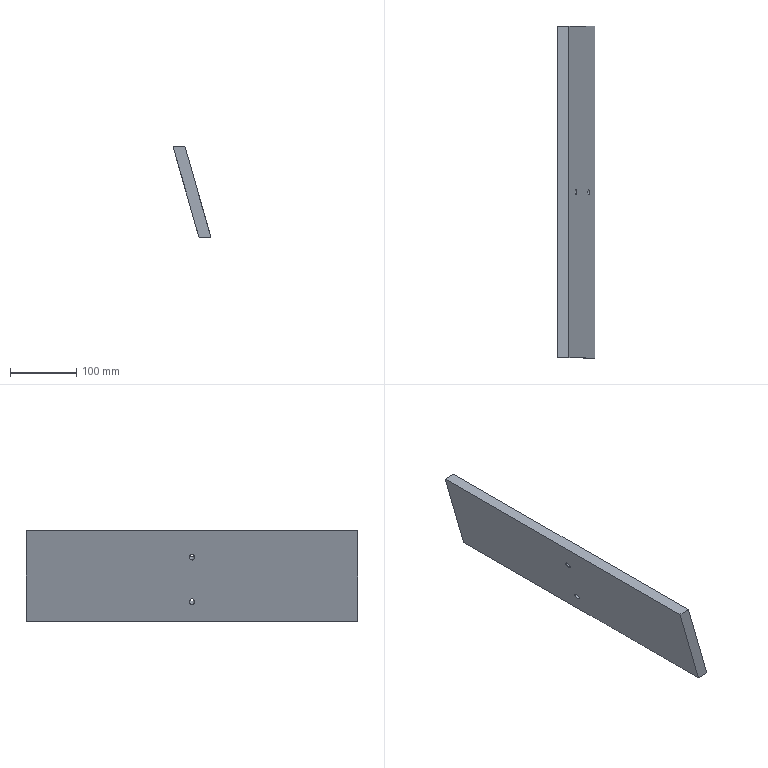Part | STEP file | Frame_top | 1 solid | 8 faces | box 57.278 x 502 x 136.98 mm | volume 1235548 mm3 | plane 6 | cylinder 2 | commonest cylinder face diameters 9 x2
STEP:
#1=CARTESIAN_POINT('',(0.,0.,0.));
#2=DIRECTION('',(0.,0.,1.));
#3=DIRECTION('',(1.,0.,0.));
#4=AXIS2_PLACEMENT_3D('',#1,#2,#3);
#5=CARTESIAN_POINT('',(-29.43,251.,71.25));
#6=VERTEX_POINT('',#5);
#7=CARTESIAN_POINT('',(-29.43,-251.,71.25));
#8=VERTEX_POINT('',#7);
#9=CARTESIAN_POINT('',(-29.43,251.,71.25));
#10=DIRECTION('',(0.,-1.,0.));
#11=VECTOR('',#10,1.);
#12=LINE('',#9,#11);
#13=CARTESIAN_POINT('',(-29.43,251.,71.25));
#14=DIRECTION('',(0.,0.,1.));
#15=DIRECTION('',(1.,0.,0.));
#16=AXIS2_PLACEMENT_3D('',#13,#14,#15);
#17=PLANE('',#16);
#18=CARTESIAN_POINT('',(0.,0.));
#19=DIRECTION('',(0.,-1.));
#20=VECTOR('',#19,1.);
#21=LINE('',#18,#20);
#22=(GEOMETRIC_REPRESENTATION_CONTEXT(2)PARAMETRIC_REPRESENTATION_CONTEXT()REPRESENTATION_CONTEXT('',''));
#23=DEFINITIONAL_REPRESENTATION('',(#21),#22);
#24=PCURVE('',#17,#23);
#25=CARTESIAN_POINT('',(9.848,251.,-65.73));
#26=DIRECTION('',(-0.9613,0.,-0.2756));
#27=DIRECTION('',(-0.2756,0.,0.9613));
#28=AXIS2_PLACEMENT_3D('',#25,#26,#27);
#29=PLANE('',#28);
#30=CARTESIAN_POINT('',(142.5,0.));
#31=DIRECTION('',(0.,-1.));
#32=VECTOR('',#31,1.);
#33=LINE('',#30,#32);
#34=(GEOMETRIC_REPRESENTATION_CONTEXT(2)PARAMETRIC_REPRESENTATION_CONTEXT()REPRESENTATION_CONTEXT('',''));
#35=DEFINITIONAL_REPRESENTATION('',(#33),#34);
#36=PCURVE('',#29,#35);
#37=SURFACE_CURVE('',#12,(#24,#36),.PCURVE_S1.);
#38=EDGE_CURVE('',#6,#8,#37,.T.);
#39=ORIENTED_EDGE('',*,*,#38,.T.);
#40=CARTESIAN_POINT('',(-11.43,-251.,71.25));
#41=VERTEX_POINT('',#40);
#42=CARTESIAN_POINT('',(-29.43,-251.,71.25));
#43=DIRECTION('',(1.,0.,0.));
#44=VECTOR('',#43,1.);
#45=LINE('',#42,#44);
#46=CARTESIAN_POINT('',(0.,-502.));
#47=DIRECTION('',(1.,0.));
#48=VECTOR('',#47,1.);
#49=LINE('',#46,#48);
#50=(GEOMETRIC_REPRESENTATION_CONTEXT(2)PARAMETRIC_REPRESENTATION_CONTEXT()REPRESENTATION_CONTEXT('',''));
#51=DEFINITIONAL_REPRESENTATION('',(#49),#50);
#52=PCURVE('',#17,#51);
#53=CARTESIAN_POINT('',(-0.7909,-251.,2.76));
#54=DIRECTION('',(0.,1.,0.));
#55=DIRECTION('',(0.,0.,1.));
#56=AXIS2_PLACEMENT_3D('',#53,#54,#55);
#57=PLANE('',#56);
#58=CARTESIAN_POINT('',(68.49,-28.639));
#59=DIRECTION('',(0.,1.));
#60=VECTOR('',#59,1.);
#61=LINE('',#58,#60);
#62=(GEOMETRIC_REPRESENTATION_CONTEXT(2)PARAMETRIC_REPRESENTATION_CONTEXT()REPRESENTATION_CONTEXT('',''));
#63=DEFINITIONAL_REPRESENTATION('',(#61),#62);
#64=PCURVE('',#57,#63);
#65=SURFACE_CURVE('',#45,(#52,#64),.PCURVE_S1.);
#66=EDGE_CURVE('',#8,#41,#65,.T.);
#67=ORIENTED_EDGE('',*,*,#66,.T.);
#68=CARTESIAN_POINT('',(-11.43,251.,71.25));
#69=VERTEX_POINT('',#68);
#70=CARTESIAN_POINT('',(-11.43,251.,71.25));
#71=DIRECTION('',(0.,-1.,0.));
#72=VECTOR('',#71,1.);
#73=LINE('',#70,#72);
#74=CARTESIAN_POINT('',(18.,0.));
#75=DIRECTION('',(0.,-1.));
#76=VECTOR('',#75,1.);
#77=LINE('',#74,#76);
#78=(GEOMETRIC_REPRESENTATION_CONTEXT(2)PARAMETRIC_REPRESENTATION_CONTEXT()REPRESENTATION_CONTEXT('',''));
#79=DEFINITIONAL_REPRESENTATION('',(#77),#78);
#80=PCURVE('',#17,#79);
#81=CARTESIAN_POINT('',(-11.43,251.,71.25));
#82=DIRECTION('',(0.9613,0.,0.2756));
#83=DIRECTION('',(0.2756,0.,-0.9613));
#84=AXIS2_PLACEMENT_3D('',#81,#82,#83);
#85=PLANE('',#84);
#86=CARTESIAN_POINT('',(0.,0.));
#87=DIRECTION('',(0.,-1.));
#88=VECTOR('',#87,1.);
#89=LINE('',#86,#88);
#90=(GEOMETRIC_REPRESENTATION_CONTEXT(2)PARAMETRIC_REPRESENTATION_CONTEXT()REPRESENTATION_CONTEXT('',''));
#91=DEFINITIONAL_REPRESENTATION('',(#89),#90);
#92=PCURVE('',#85,#91);
#93=SURFACE_CURVE('',#73,(#80,#92),.PCURVE_S1.);
#94=EDGE_CURVE('',#69,#41,#93,.T.);
#95=ORIENTED_EDGE('',*,*,#94,.F.);
#96=CARTESIAN_POINT('',(-29.43,251.,71.25));
#97=DIRECTION('',(1.,0.,0.));
#98=VECTOR('',#97,1.);
#99=LINE('',#96,#98);
#100=CARTESIAN_POINT('',(0.,0.));
#101=DIRECTION('',(1.,0.));
#102=VECTOR('',#101,1.);
#103=LINE('',#100,#102);
#104=(GEOMETRIC_REPRESENTATION_CONTEXT(2)PARAMETRIC_REPRESENTATION_CONTEXT()REPRESENTATION_CONTEXT('',''));
#105=DEFINITIONAL_REPRESENTATION('',(#103),#104);
#106=PCURVE('',#17,#105);
#107=CARTESIAN_POINT('',(-0.7909,251.,2.76));
#108=DIRECTION('',(0.,1.,0.));
#109=DIRECTION('',(0.,0.,1.));
#110=AXIS2_PLACEMENT_3D('',#107,#108,#109);
#111=PLANE('',#110);
#112=CARTESIAN_POINT('',(68.49,-28.639));
#113=DIRECTION('',(0.,1.));
#114=VECTOR('',#113,1.);
#115=LINE('',#112,#114);
#116=(GEOMETRIC_REPRESENTATION_CONTEXT(2)PARAMETRIC_REPRESENTATION_CONTEXT()REPRESENTATION_CONTEXT('',''));
#117=DEFINITIONAL_REPRESENTATION('',(#115),#116);
#118=PCURVE('',#111,#117);
#119=SURFACE_CURVE('',#99,(#106,#118),.PCURVE_S1.);
#120=EDGE_CURVE('',#6,#69,#119,.T.);
#121=ORIENTED_EDGE('',*,*,#120,.F.);
#122=EDGE_LOOP('',(#39,#67,#95,#121));
#123=FACE_BOUND('',#122,.T.);
#124=ADVANCED_FACE('',(#123),#17,.T.);
#125=CARTESIAN_POINT('',(9.848,251.,-65.73));
#126=VERTEX_POINT('',#125);
#127=CARTESIAN_POINT('',(9.848,-251.,-65.73));
#128=VERTEX_POINT('',#127);
#129=CARTESIAN_POINT('',(9.848,251.,-65.73));
#130=DIRECTION('',(0.,-1.,0.));
#131=VECTOR('',#130,1.);
#132=LINE('',#129,#131);
#133=CARTESIAN_POINT('',(0.,0.));
#134=DIRECTION('',(0.,-1.));
#135=VECTOR('',#134,1.);
#136=LINE('',#133,#135);
#137=(GEOMETRIC_REPRESENTATION_CONTEXT(2)PARAMETRIC_REPRESENTATION_CONTEXT()REPRESENTATION_CONTEXT('',''));
#138=DEFINITIONAL_REPRESENTATION('',(#136),#137);
#139=PCURVE('',#29,#138);
#140=CARTESIAN_POINT('',(27.848,251.,-65.73));
#141=DIRECTION('',(0.,0.,-1.));
#142=DIRECTION('',(-1.,0.,0.));
#143=AXIS2_PLACEMENT_3D('',#140,#141,#142);
#144=PLANE('',#143);
#145=CARTESIAN_POINT('',(18.,0.));
#146=DIRECTION('',(0.,-1.));
#147=VECTOR('',#146,1.);
#148=LINE('',#145,#147);
#149=(GEOMETRIC_REPRESENTATION_CONTEXT(2)PARAMETRIC_REPRESENTATION_CONTEXT()REPRESENTATION_CONTEXT('',''));
#150=DEFINITIONAL_REPRESENTATION('',(#148),#149);
#151=PCURVE('',#144,#150);
#152=SURFACE_CURVE('',#132,(#139,#151),.PCURVE_S1.);
#153=EDGE_CURVE('',#126,#128,#152,.T.);
#154=ORIENTED_EDGE('',*,*,#153,.T.);
#155=CARTESIAN_POINT('',(9.848,-251.,-65.73));
#156=DIRECTION('',(-0.2756,0.,0.9613));
#157=VECTOR('',#156,1.);
#158=LINE('',#155,#157);
#159=CARTESIAN_POINT('',(0.,-502.));
#160=DIRECTION('',(1.,0.));
#161=VECTOR('',#160,1.);
#162=LINE('',#159,#161);
#163=(GEOMETRIC_REPRESENTATION_CONTEXT(2)PARAMETRIC_REPRESENTATION_CONTEXT()REPRESENTATION_CONTEXT('',''));
#164=DEFINITIONAL_REPRESENTATION('',(#162),#163);
#165=PCURVE('',#29,#164);
#166=CARTESIAN_POINT('',(-68.49,10.639));
#167=DIRECTION('',(0.9613,-0.2756));
#168=VECTOR('',#167,1.);
#169=LINE('',#166,#168);
#170=(GEOMETRIC_REPRESENTATION_CONTEXT(2)PARAMETRIC_REPRESENTATION_CONTEXT()REPRESENTATION_CONTEXT('',''));
#171=DEFINITIONAL_REPRESENTATION('',(#169),#170);
#172=PCURVE('',#57,#171);
#173=SURFACE_CURVE('',#158,(#165,#172),.PCURVE_S1.);
#174=EDGE_CURVE('',#128,#8,#173,.T.);
#175=ORIENTED_EDGE('',*,*,#174,.T.);
#176=ORIENTED_EDGE('',*,*,#38,.F.);
#177=CARTESIAN_POINT('',(9.848,251.,-65.73));
#178=DIRECTION('',(-0.2756,0.,0.9613));
#179=VECTOR('',#178,1.);
#180=LINE('',#177,#179);
#181=CARTESIAN_POINT('',(0.,0.));
#182=DIRECTION('',(1.,0.));
#183=VECTOR('',#182,1.);
#184=LINE('',#181,#183);
#185=(GEOMETRIC_REPRESENTATION_CONTEXT(2)PARAMETRIC_REPRESENTATION_CONTEXT()REPRESENTATION_CONTEXT('',''));
#186=DEFINITIONAL_REPRESENTATION('',(#184),#185);
#187=PCURVE('',#29,#186);
#188=CARTESIAN_POINT('',(-68.49,10.639));
#189=DIRECTION('',(0.9613,-0.2756));
#190=VECTOR('',#189,1.);
#191=LINE('',#188,#190);
#192=(GEOMETRIC_REPRESENTATION_CONTEXT(2)PARAMETRIC_REPRESENTATION_CONTEXT()REPRESENTATION_CONTEXT('',''));
#193=DEFINITIONAL_REPRESENTATION('',(#191),#192);
#194=PCURVE('',#111,#193);
#195=SURFACE_CURVE('',#180,(#187,#194),.PCURVE_S1.);
#196=EDGE_CURVE('',#126,#6,#195,.T.);
#197=ORIENTED_EDGE('',*,*,#196,.F.);
#198=EDGE_LOOP('',(#154,#175,#176,#197));
#199=FACE_BOUND('',#198,.T.);
#200=CARTESIAN_POINT('',(-16.723,0.,26.934));
#201=VERTEX_POINT('',#200);
#202=CARTESIAN_POINT('',(-17.963,0.,31.26));
#203=DIRECTION('',(-0.9613,0.,-0.2756));
#204=DIRECTION('',(0.2756,0.,-0.9613));
#205=AXIS2_PLACEMENT_3D('',#202,#203,#204);
#206=CIRCLE('',#205,4.5);
#207=CARTESIAN_POINT('',(100.898,-251.));
#208=DIRECTION('',(-1.,0.));
#209=AXIS2_PLACEMENT_2D('',#207,#208);
#210=CIRCLE('',#209,4.5);
#211=(GEOMETRIC_REPRESENTATION_CONTEXT(2)PARAMETRIC_REPRESENTATION_CONTEXT()REPRESENTATION_CONTEXT('',''));
#212=DEFINITIONAL_REPRESENTATION('',(#210),#211);
#213=PCURVE('',#29,#212);
#214=CARTESIAN_POINT('',(-1.331,0.,36.029));
#215=DIRECTION('',(-0.9613,0.,-0.2756));
#216=DIRECTION('',(0.2756,0.,-0.9613));
#217=AXIS2_PLACEMENT_3D('',#214,#215,#216);
#218=CYLINDRICAL_SURFACE('',#217,4.5);
#219=CARTESIAN_POINT('',(0.,17.303));
#220=DIRECTION('',(1.,0.));
#221=VECTOR('',#220,1.);
#222=LINE('',#219,#221);
#223=(GEOMETRIC_REPRESENTATION_CONTEXT(2)PARAMETRIC_REPRESENTATION_CONTEXT()REPRESENTATION_CONTEXT('',''));
#224=DEFINITIONAL_REPRESENTATION('',(#222),#223);
#225=PCURVE('',#218,#224);
#226=SURFACE_CURVE('',#206,(#213,#225),.PCURVE_S1.);
#227=EDGE_CURVE('',#201,#201,#226,.T.);
#228=ORIENTED_EDGE('',*,*,#227,.F.);
#229=EDGE_LOOP('',(#228));
#230=FACE_BOUND('',#229,.T.);
#231=CARTESIAN_POINT('',(2.572,0.,-40.354));
#232=VERTEX_POINT('',#231);
#233=CARTESIAN_POINT('',(1.332,0.,-36.029));
#234=DIRECTION('',(-0.9613,0.,-0.2756));
#235=DIRECTION('',(0.2756,0.,-0.9613));
#236=AXIS2_PLACEMENT_3D('',#233,#234,#235);
#237=CIRCLE('',#236,4.5);
#238=CARTESIAN_POINT('',(30.898,-251.));
#239=DIRECTION('',(-1.,0.));
#240=AXIS2_PLACEMENT_2D('',#238,#239);
#241=CIRCLE('',#240,4.5);
#242=(GEOMETRIC_REPRESENTATION_CONTEXT(2)PARAMETRIC_REPRESENTATION_CONTEXT()REPRESENTATION_CONTEXT('',''));
#243=DEFINITIONAL_REPRESENTATION('',(#241),#242);
#244=PCURVE('',#29,#243);
#245=CARTESIAN_POINT('',(17.964,0.,-31.259));
#246=DIRECTION('',(-0.9613,0.,-0.2756));
#247=DIRECTION('',(0.2756,0.,-0.9613));
#248=AXIS2_PLACEMENT_3D('',#245,#246,#247);
#249=CYLINDRICAL_SURFACE('',#248,4.5);
#250=CARTESIAN_POINT('',(0.,17.303));
#251=DIRECTION('',(1.,0.));
#252=VECTOR('',#251,1.);
#253=LINE('',#250,#252);
#254=(GEOMETRIC_REPRESENTATION_CONTEXT(2)PARAMETRIC_REPRESENTATION_CONTEXT()REPRESENTATION_CONTEXT('',''));
#255=DEFINITIONAL_REPRESENTATION('',(#253),#254);
#256=PCURVE('',#249,#255);
#257=SURFACE_CURVE('',#237,(#244,#256),.PCURVE_S1.);
#258=EDGE_CURVE('',#232,#232,#257,.T.);
#259=ORIENTED_EDGE('',*,*,#258,.F.);
#260=EDGE_LOOP('',(#259));
#261=FACE_BOUND('',#260,.T.);
#262=ADVANCED_FACE('',(#199,#230,#261),#29,.T.);
#263=ORIENTED_EDGE('',*,*,#94,.T.);
#264=CARTESIAN_POINT('',(27.848,-251.,-65.73));
#265=VERTEX_POINT('',#264);
#266=CARTESIAN_POINT('',(-11.43,-251.,71.25));
#267=DIRECTION('',(0.2756,0.,-0.9613));
#268=VECTOR('',#267,1.);
#269=LINE('',#266,#268);
#270=CARTESIAN_POINT('',(0.,-502.));
#271=DIRECTION('',(1.,0.));
#272=VECTOR('',#271,1.);
#273=LINE('',#270,#272);
#274=(GEOMETRIC_REPRESENTATION_CONTEXT(2)PARAMETRIC_REPRESENTATION_CONTEXT()REPRESENTATION_CONTEXT('',''));
#275=DEFINITIONAL_REPRESENTATION('',(#273),#274);
#276=PCURVE('',#85,#275);
#277=CARTESIAN_POINT('',(68.49,-10.639));
#278=DIRECTION('',(-0.9613,0.2756));
#279=VECTOR('',#278,1.);
#280=LINE('',#277,#279);
#281=(GEOMETRIC_REPRESENTATION_CONTEXT(2)PARAMETRIC_REPRESENTATION_CONTEXT()REPRESENTATION_CONTEXT('',''));
#282=DEFINITIONAL_REPRESENTATION('',(#280),#281);
#283=PCURVE('',#57,#282);
#284=SURFACE_CURVE('',#269,(#276,#283),.PCURVE_S1.);
#285=EDGE_CURVE('',#41,#265,#284,.T.);
#286=ORIENTED_EDGE('',*,*,#285,.T.);
#287=CARTESIAN_POINT('',(27.848,251.,-65.73));
#288=VERTEX_POINT('',#287);
#289=CARTESIAN_POINT('',(27.848,251.,-65.73));
#290=DIRECTION('',(0.,-1.,0.));
#291=VECTOR('',#290,1.);
#292=LINE('',#289,#291);
#293=CARTESIAN_POINT('',(142.5,0.));
#294=DIRECTION('',(0.,-1.));
#295=VECTOR('',#294,1.);
#296=LINE('',#293,#295);
#297=(GEOMETRIC_REPRESENTATION_CONTEXT(2)PARAMETRIC_REPRESENTATION_CONTEXT()REPRESENTATION_CONTEXT('',''));
#298=DEFINITIONAL_REPRESENTATION('',(#296),#297);
#299=PCURVE('',#85,#298);
#300=CARTESIAN_POINT('',(0.,0.));
#301=DIRECTION('',(0.,-1.));
#302=VECTOR('',#301,1.);
#303=LINE('',#300,#302);
#304=(GEOMETRIC_REPRESENTATION_CONTEXT(2)PARAMETRIC_REPRESENTATION_CONTEXT()REPRESENTATION_CONTEXT('',''));
#305=DEFINITIONAL_REPRESENTATION('',(#303),#304);
#306=PCURVE('',#144,#305);
#307=SURFACE_CURVE('',#292,(#299,#306),.PCURVE_S1.);
#308=EDGE_CURVE('',#288,#265,#307,.T.);
#309=ORIENTED_EDGE('',*,*,#308,.F.);
#310=CARTESIAN_POINT('',(-11.43,251.,71.25));
#311=DIRECTION('',(0.2756,0.,-0.9613));
#312=VECTOR('',#311,1.);
#313=LINE('',#310,#312);
#314=CARTESIAN_POINT('',(0.,0.));
#315=DIRECTION('',(1.,0.));
#316=VECTOR('',#315,1.);
#317=LINE('',#314,#316);
#318=(GEOMETRIC_REPRESENTATION_CONTEXT(2)PARAMETRIC_REPRESENTATION_CONTEXT()REPRESENTATION_CONTEXT('',''));
#319=DEFINITIONAL_REPRESENTATION('',(#317),#318);
#320=PCURVE('',#85,#319);
#321=CARTESIAN_POINT('',(68.49,-10.639));
#322=DIRECTION('',(-0.9613,0.2756));
#323=VECTOR('',#322,1.);
#324=LINE('',#321,#323);
#325=(GEOMETRIC_REPRESENTATION_CONTEXT(2)PARAMETRIC_REPRESENTATION_CONTEXT()REPRESENTATION_CONTEXT('',''));
#326=DEFINITIONAL_REPRESENTATION('',(#324),#325);
#327=PCURVE('',#111,#326);
#328=SURFACE_CURVE('',#313,(#320,#327),.PCURVE_S1.);
#329=EDGE_CURVE('',#69,#288,#328,.T.);
#330=ORIENTED_EDGE('',*,*,#329,.F.);
#331=EDGE_LOOP('',(#263,#286,#309,#330));
#332=FACE_BOUND('',#331,.T.);
#333=CARTESIAN_POINT('',(-0.09017,0.,31.703));
#334=VERTEX_POINT('',#333);
#335=CARTESIAN_POINT('',(-1.331,0.,36.029));
#336=DIRECTION('',(0.9613,0.,0.2756));
#337=DIRECTION('',(0.2756,0.,-0.9613));
#338=AXIS2_PLACEMENT_3D('',#335,#336,#337);
#339=CIRCLE('',#338,4.5);
#340=CARTESIAN_POINT('',(36.64,-251.));
#341=DIRECTION('',(1.,0.));
#342=AXIS2_PLACEMENT_2D('',#340,#341);
#343=CIRCLE('',#342,4.5);
#344=(GEOMETRIC_REPRESENTATION_CONTEXT(2)PARAMETRIC_REPRESENTATION_CONTEXT()REPRESENTATION_CONTEXT('',''));
#345=DEFINITIONAL_REPRESENTATION('',(#343),#344);
#346=PCURVE('',#85,#345);
#347=CARTESIAN_POINT('',(6.283,0.));
#348=DIRECTION('',(-1.,0.));
#349=VECTOR('',#348,1.);
#350=LINE('',#347,#349);
#351=(GEOMETRIC_REPRESENTATION_CONTEXT(2)PARAMETRIC_REPRESENTATION_CONTEXT()REPRESENTATION_CONTEXT('',''));
#352=DEFINITIONAL_REPRESENTATION('',(#350),#351);
#353=PCURVE('',#218,#352);
#354=SURFACE_CURVE('',#339,(#346,#353),.PCURVE_S1.);
#355=EDGE_CURVE('',#334,#334,#354,.T.);
#356=ORIENTED_EDGE('',*,*,#355,.F.);
#357=EDGE_LOOP('',(#356));
#358=FACE_BOUND('',#357,.T.);
#359=CARTESIAN_POINT('',(19.204,0.,-35.585));
#360=VERTEX_POINT('',#359);
#361=CARTESIAN_POINT('',(17.964,0.,-31.259));
#362=DIRECTION('',(0.9613,0.,0.2756));
#363=DIRECTION('',(0.2756,0.,-0.9613));
#364=AXIS2_PLACEMENT_3D('',#361,#362,#363);
#365=CIRCLE('',#364,4.5);
#366=CARTESIAN_POINT('',(106.64,-251.));
#367=DIRECTION('',(1.,0.));
#368=AXIS2_PLACEMENT_2D('',#366,#367);
#369=CIRCLE('',#368,4.5);
#370=(GEOMETRIC_REPRESENTATION_CONTEXT(2)PARAMETRIC_REPRESENTATION_CONTEXT()REPRESENTATION_CONTEXT('',''));
#371=DEFINITIONAL_REPRESENTATION('',(#369),#370);
#372=PCURVE('',#85,#371);
#373=CARTESIAN_POINT('',(6.283,0.));
#374=DIRECTION('',(-1.,0.));
#375=VECTOR('',#374,1.);
#376=LINE('',#373,#375);
#377=(GEOMETRIC_REPRESENTATION_CONTEXT(2)PARAMETRIC_REPRESENTATION_CONTEXT()REPRESENTATION_CONTEXT('',''));
#378=DEFINITIONAL_REPRESENTATION('',(#376),#377);
#379=PCURVE('',#249,#378);
#380=SURFACE_CURVE('',#365,(#372,#379),.PCURVE_S1.);
#381=EDGE_CURVE('',#360,#360,#380,.T.);
#382=ORIENTED_EDGE('',*,*,#381,.F.);
#383=EDGE_LOOP('',(#382));
#384=FACE_BOUND('',#383,.T.);
#385=ADVANCED_FACE('',(#332,#358,#384),#85,.T.);
#386=ORIENTED_EDGE('',*,*,#120,.T.);
#387=ORIENTED_EDGE('',*,*,#329,.T.);
#388=CARTESIAN_POINT('',(27.848,251.,-65.73));
#389=DIRECTION('',(-1.,0.,0.));
#390=VECTOR('',#389,1.);
#391=LINE('',#388,#390);
#392=CARTESIAN_POINT('',(-68.49,28.639));
#393=DIRECTION('',(0.,-1.));
#394=VECTOR('',#393,1.);
#395=LINE('',#392,#394);
#396=(GEOMETRIC_REPRESENTATION_CONTEXT(2)PARAMETRIC_REPRESENTATION_CONTEXT()REPRESENTATION_CONTEXT('',''));
#397=DEFINITIONAL_REPRESENTATION('',(#395),#396);
#398=PCURVE('',#111,#397);
#399=CARTESIAN_POINT('',(0.,0.));
#400=DIRECTION('',(1.,0.));
#401=VECTOR('',#400,1.);
#402=LINE('',#399,#401);
#403=(GEOMETRIC_REPRESENTATION_CONTEXT(2)PARAMETRIC_REPRESENTATION_CONTEXT()REPRESENTATION_CONTEXT('',''));
#404=DEFINITIONAL_REPRESENTATION('',(#402),#403);
#405=PCURVE('',#144,#404);
#406=SURFACE_CURVE('',#391,(#398,#405),.PCURVE_S1.);
#407=EDGE_CURVE('',#288,#126,#406,.T.);
#408=ORIENTED_EDGE('',*,*,#407,.T.);
#409=ORIENTED_EDGE('',*,*,#196,.T.);
#410=EDGE_LOOP('',(#386,#387,#408,#409));
#411=FACE_BOUND('',#410,.T.);
#412=ADVANCED_FACE('',(#411),#111,.T.);
#413=ORIENTED_EDGE('',*,*,#66,.T.);
#414=ORIENTED_EDGE('',*,*,#285,.T.);
#415=CARTESIAN_POINT('',(27.848,-251.,-65.73));
#416=DIRECTION('',(-1.,0.,0.));
#417=VECTOR('',#416,1.);
#418=LINE('',#415,#417);
#419=CARTESIAN_POINT('',(-68.49,28.639));
#420=DIRECTION('',(0.,-1.));
#421=VECTOR('',#420,1.);
#422=LINE('',#419,#421);
#423=(GEOMETRIC_REPRESENTATION_CONTEXT(2)PARAMETRIC_REPRESENTATION_CONTEXT()REPRESENTATION_CONTEXT('',''));
#424=DEFINITIONAL_REPRESENTATION('',(#422),#423);
#425=PCURVE('',#57,#424);
#426=CARTESIAN_POINT('',(0.,-502.));
#427=DIRECTION('',(1.,0.));
#428=VECTOR('',#427,1.);
#429=LINE('',#426,#428);
#430=(GEOMETRIC_REPRESENTATION_CONTEXT(2)PARAMETRIC_REPRESENTATION_CONTEXT()REPRESENTATION_CONTEXT('',''));
#431=DEFINITIONAL_REPRESENTATION('',(#429),#430);
#432=PCURVE('',#144,#431);
#433=SURFACE_CURVE('',#418,(#425,#432),.PCURVE_S1.);
#434=EDGE_CURVE('',#265,#128,#433,.T.);
#435=ORIENTED_EDGE('',*,*,#434,.T.);
#436=ORIENTED_EDGE('',*,*,#174,.T.);
#437=EDGE_LOOP('',(#413,#414,#435,#436));
#438=FACE_BOUND('',#437,.F.);
#439=ADVANCED_FACE('',(#438),#57,.F.);
#440=ORIENTED_EDGE('',*,*,#308,.T.);
#441=ORIENTED_EDGE('',*,*,#434,.T.);
#442=ORIENTED_EDGE('',*,*,#153,.F.);
#443=ORIENTED_EDGE('',*,*,#407,.F.);
#444=EDGE_LOOP('',(#440,#441,#442,#443));
#445=FACE_BOUND('',#444,.T.);
#446=ADVANCED_FACE('',(#445),#144,.T.);
#447=ORIENTED_EDGE('',*,*,#227,.F.);
#448=CARTESIAN_POINT('',(-0.09017,0.,31.703));
#449=DIRECTION('',(-0.9613,0.,-0.2756));
#450=VECTOR('',#449,1.);
#451=LINE('',#448,#450);
#452=CARTESIAN_POINT('',(0.,0.));
#453=DIRECTION('',(0.,1.));
#454=VECTOR('',#453,1.);
#455=LINE('',#452,#454);
#456=(GEOMETRIC_REPRESENTATION_CONTEXT(2)PARAMETRIC_REPRESENTATION_CONTEXT()REPRESENTATION_CONTEXT('',''));
#457=DEFINITIONAL_REPRESENTATION('',(#455),#456);
#458=PCURVE('',#218,#457);
#459=CARTESIAN_POINT('',(6.283,0.));
#460=DIRECTION('',(0.,1.));
#461=VECTOR('',#460,1.);
#462=LINE('',#459,#461);
#463=(GEOMETRIC_REPRESENTATION_CONTEXT(2)PARAMETRIC_REPRESENTATION_CONTEXT()REPRESENTATION_CONTEXT('',''));
#464=DEFINITIONAL_REPRESENTATION('',(#462),#463);
#465=PCURVE('',#218,#464);
#466=SEAM_CURVE('',#451,(#458,#465),.PCURVE_S1.);
#467=EDGE_CURVE('',#334,#201,#466,.T.);
#468=ORIENTED_EDGE('',*,*,#467,.F.);
#469=ORIENTED_EDGE('',*,*,#355,.F.);
#470=ORIENTED_EDGE('',*,*,#467,.T.);
#471=EDGE_LOOP('',(#447,#468,#469,#470));
#472=FACE_BOUND('',#471,.F.);
#473=ADVANCED_FACE('',(#472),#218,.F.);
#474=ORIENTED_EDGE('',*,*,#258,.F.);
#475=CARTESIAN_POINT('',(19.204,0.,-35.585));
#476=DIRECTION('',(-0.9613,0.,-0.2756));
#477=VECTOR('',#476,1.);
#478=LINE('',#475,#477);
#479=CARTESIAN_POINT('',(0.,0.));
#480=DIRECTION('',(0.,1.));
#481=VECTOR('',#480,1.);
#482=LINE('',#479,#481);
#483=(GEOMETRIC_REPRESENTATION_CONTEXT(2)PARAMETRIC_REPRESENTATION_CONTEXT()REPRESENTATION_CONTEXT('',''));
#484=DEFINITIONAL_REPRESENTATION('',(#482),#483);
#485=PCURVE('',#249,#484);
#486=CARTESIAN_POINT('',(6.283,0.));
#487=DIRECTION('',(0.,1.));
#488=VECTOR('',#487,1.);
#489=LINE('',#486,#488);
#490=(GEOMETRIC_REPRESENTATION_CONTEXT(2)PARAMETRIC_REPRESENTATION_CONTEXT()REPRESENTATION_CONTEXT('',''));
#491=DEFINITIONAL_REPRESENTATION('',(#489),#490);
#492=PCURVE('',#249,#491);
#493=SEAM_CURVE('',#478,(#485,#492),.PCURVE_S1.);
#494=EDGE_CURVE('',#360,#232,#493,.T.);
#495=ORIENTED_EDGE('',*,*,#494,.F.);
#496=ORIENTED_EDGE('',*,*,#381,.F.);
#497=ORIENTED_EDGE('',*,*,#494,.T.);
#498=EDGE_LOOP('',(#474,#495,#496,#497));
#499=FACE_BOUND('',#498,.F.);
#500=ADVANCED_FACE('',(#499),#249,.F.);
#501=CLOSED_SHELL('',(#124,#262,#385,#412,#439,#446,#473,#500));
#502=MANIFOLD_SOLID_BREP('',#501);
#503=(LENGTH_UNIT()NAMED_UNIT(*)SI_UNIT(.MILLI.,.METRE.));
#504=UNCERTAINTY_MEASURE_WITH_UNIT(LENGTH_MEASURE(0.0000001),#503,'','');
#505=(NAMED_UNIT(*)PLANE_ANGLE_UNIT()SI_UNIT($,.RADIAN.));
#506=(NAMED_UNIT(*)SI_UNIT($,.STERADIAN.)SOLID_ANGLE_UNIT());
#507=(GEOMETRIC_REPRESENTATION_CONTEXT(3)GLOBAL_UNCERTAINTY_ASSIGNED_CONTEXT((#504))GLOBAL_UNIT_ASSIGNED_CONTEXT((#503,#505,#506))REPRESENTATION_CONTEXT('',''));
#508=ADVANCED_BREP_SHAPE_REPRESENTATION('',(#4,#502),#507);